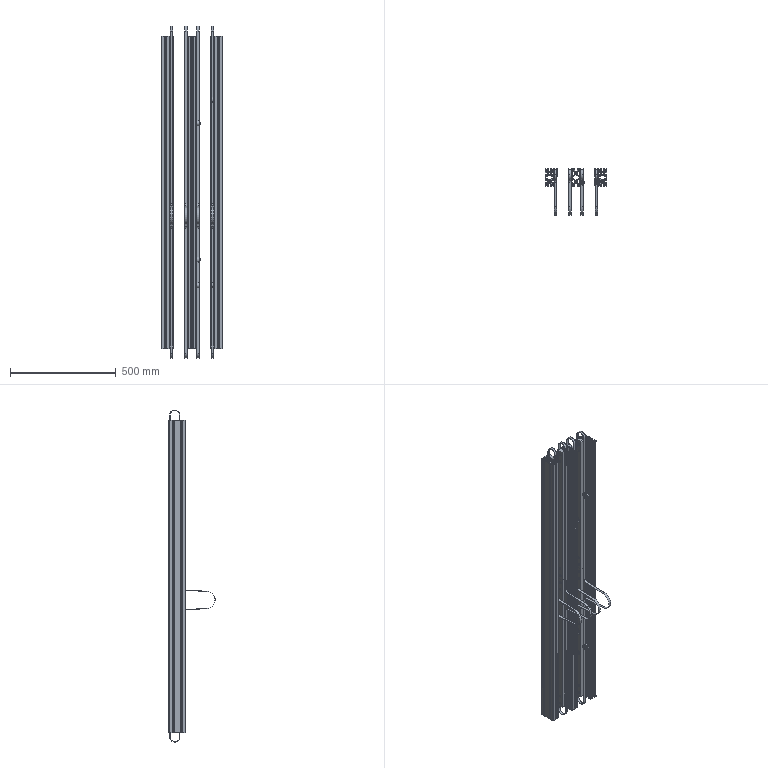Part | NX | features BREP 10 | 61 solids | 2055 faces | box 290 x 217.9 x 1568 mm | volume 8057447 mm3 | plane 787 | cylinder 752 | cone 364 | torus 152 | commonest cylinder face diameters 2 x124 8 x98 3.3 x64 0.76 x60 11 x42 10.4 x40